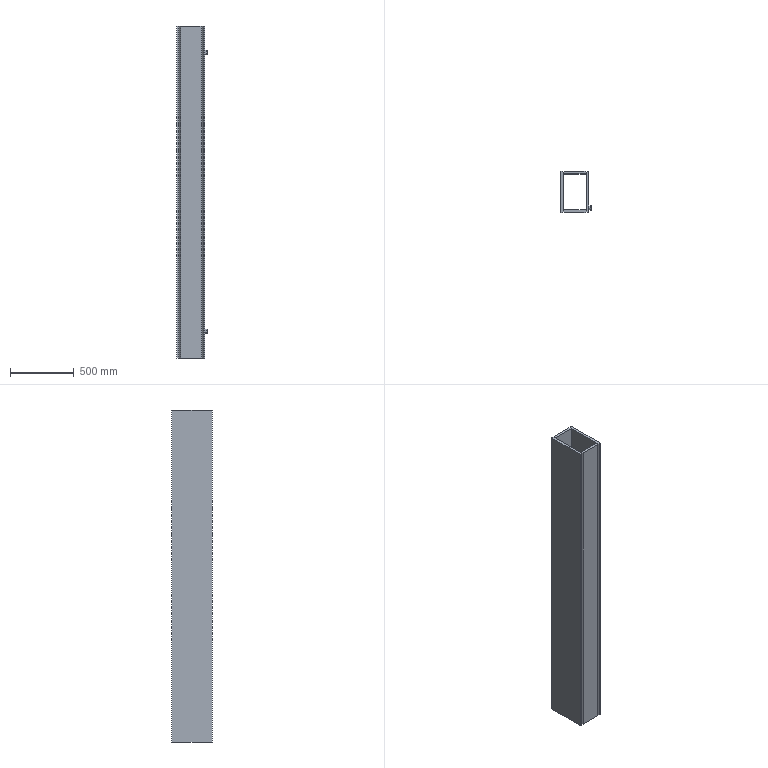Part | STEP file | Rectangular tube | 6 solids | 56 faces | box 239 x 320 x 2600 mm | volume 50963884 mm3 | plane 48 | cylinder 8 | commonest cylinder face diameters 17.5 x4 21 x4